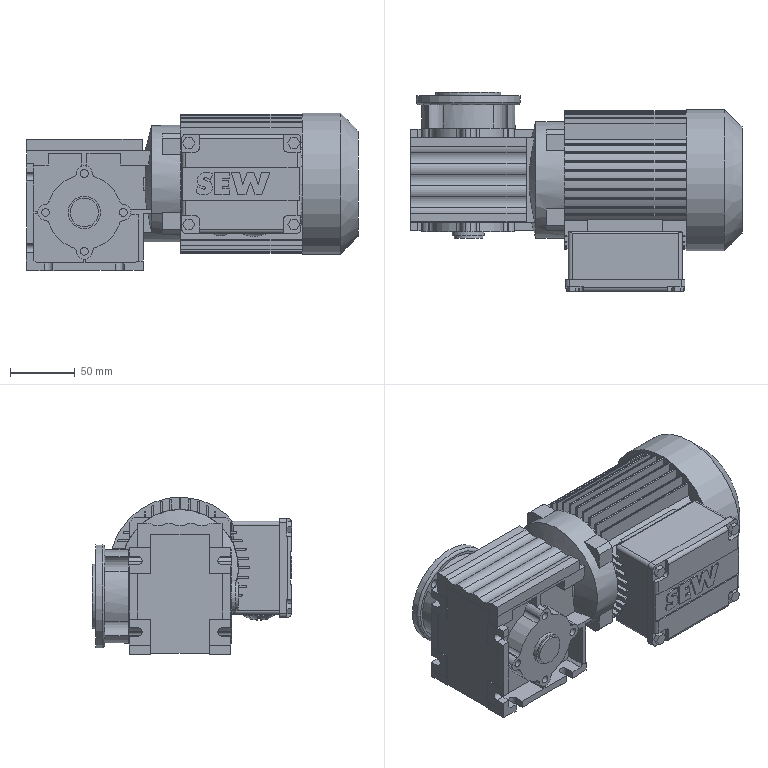Part | STEP file | 1_29 | 7 solids | 867 faces | box 256 x 153.5 x 121.5 mm | volume 2048036 mm3 | plane 550 | cylinder 305 | cone 9 | sphere 2 | torus 1 | commonest cylinder face diameters 1 x90 84 x44 0.1 x29 6 x25 2 x19 8 x16